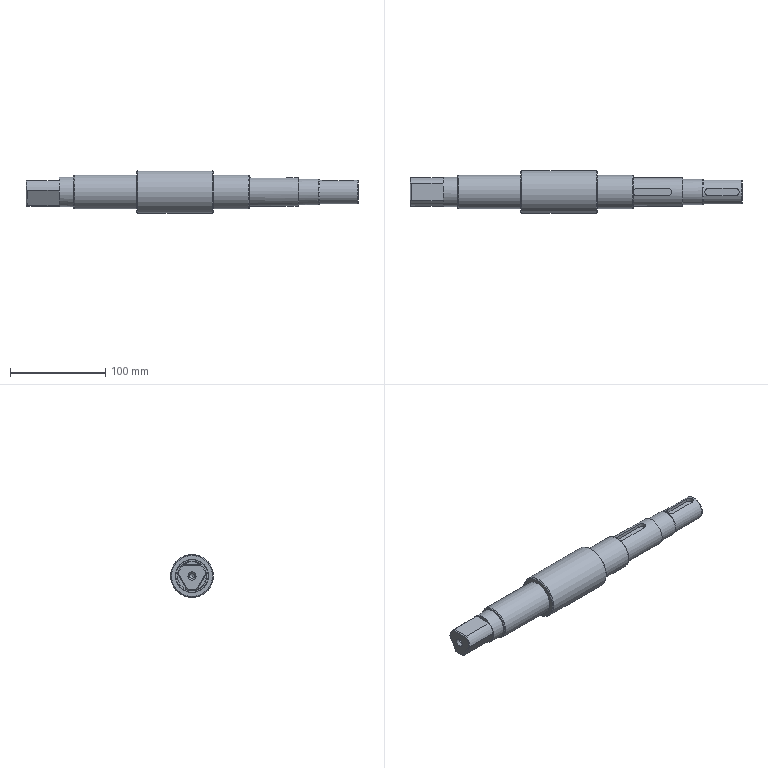NC program | NX | posted with a generic post | part box 348.4 x 45 x 45 mm
Whole program:
N10 G17 G21 G94 G90
(刀补4 , TOOL : D4)
N12 T04 M6
N14 G54
N16 G17 G0 G90 X104.872 Y0.433 B0. C0. S4500 M3
N18 G43 Z30. H4
N20 Z-6.508
N22 G94 G1 X102.135 Z-6.652 F1000.
N24 X101.983 Y0.386 Z-6.66
N26 X101.822 Y0.23 Z-6.672
N28 X101.758 Y0.016 Z-6.684
N30 X101.806 Y-0.203 Z-6.695
N32 X101.925 Y-0.347 Z-6.705
N34 X102.106 Y-0.433 Z-6.716
N36 X111.836 Z-7.225
N38 X111.853 Y-0.422 Z-7.226
N40 X112.036 Y-0.414 Z-7.236
N42 X112.09 Y-0.412 Z-7.239
N44 X112.197 Y-0.413 Z-7.245
N46 X112.295 Y-0.411 Z-7.25
N48 X112.388 Y-0.38 Z-7.255
N50 X112.463 Y-0.354 Z-7.259
N52 X112.485 Y-0.338 Z-7.26
N54 X112.533 Y-0.275 Z-7.265
N56 X112.592 Y-0.2 Z-7.27
N58 X112.638 Y0. Z-7.28
N60 X112.592 Y0.199 Z-7.291
N62 X112.534 Y0.274 Z-7.296
N64 X112.48 Y0.329 Z-7.3
N66 X112.429 Y0.365 Z-7.303
N68 X112.196 Y0.433 Z-7.316
N70 X107.299 Z-7.573
N72 G41 X107.2 Y0.45 D4
N74 X102.2 F1650.
N76 G3 X101.75 Y0. R0.45
N78 X102.2 Y-0.45 R0.45
N80 G1 X111.841
N82 X111.858 Y-0.439
N84 X112.037 Y-0.432
N86 X112.09 Y-0.43
N88 X112.198
N90 X112.299 Y-0.431
N92 X112.394 Y-0.396
N94 X112.457 Y-0.378
N96 X112.51 Y-0.34
N98 X112.547 Y-0.285
N100 G3 X112.547 Y0.285 R0.462
N102 G1 X112.491 Y0.342
N104 X112.437 Y0.381
N106 X112.201 Y0.45
N108 X107.2
N110 X103.512 Z-7.637
N112 X102.2
N114 G3 X101.75 Y0. R0.45
N116 X102.2 Y-0.45 R0.45
N118 G1 X111.841
N120 X111.858 Y-0.439
N122 X112.037 Y-0.432
N124 X112.09 Y-0.43
N126 X112.198
N128 X112.299 Y-0.431
N130 X112.394 Y-0.396
N132 X112.457 Y-0.378
N134 X112.51 Y-0.34
N136 X112.547 Y-0.285
N138 G3 X112.547 Y0.285 R0.462
N140 G1 X112.491 Y0.342
N142 X112.437 Y0.381
N144 X112.201 Y0.45
N146 X107.2
N148 X103.512 Z-7.701
N150 X102.2
N152 G3 X101.75 Y0. R0.45
N154 X102.2 Y-0.45 R0.45
N156 G1 X111.841
N158 X111.858 Y-0.439
N160 X112.037 Y-0.432
N162 X112.09 Y-0.43
N164 X112.198
N166 X112.299 Y-0.431
N168 X112.394 Y-0.396
N170 X112.457 Y-0.378
N172 X112.51 Y-0.34
N174 X112.547 Y-0.285
N176 G3 X112.547 Y0.285 R0.462
N178 G1 X112.491 Y0.342
N180 X112.437 Y0.381
N182 X112.201 Y0.45
N184 X107.2
N186 X103.512 Z-7.766
N188 X102.2
N190 G3 X101.75 Y0. R0.45
N192 X102.2 Y-0.45 R0.45
N194 G1 X111.841
N196 X111.858 Y-0.439
N198 X112.037 Y-0.431
N200 X112.09 Y-0.43
N202 X112.198
N204 X112.299 Y-0.431
N206 X112.394 Y-0.396
N208 X112.457 Y-0.378
N210 X112.51 Y-0.34
N212 X112.547 Y-0.285
N214 G3 X112.547 Y0.285 R0.462
N216 G1 X112.491 Y0.342
N218 X112.437 Y0.381
N220 X112.201 Y0.45
N222 X107.2
N224 X103.512 Z-7.83
N226 X102.2
N228 G3 X101.75 Y0. R0.45
N230 X102.2 Y-0.45 R0.45
N232 G1 X111.841
N234 X111.852 Y-0.432
N236 X111.873 Y-0.438
N238 X112.238 Y-0.431
N240 X112.394 Y-0.396
N242 X112.457 Y-0.378
N244 X112.51 Y-0.34
N246 X112.547 Y-0.285
N248 G3 X112.563 Y0.265 R0.467
N250 G1 X112.483 Y0.348
N252 X112.437 Y0.381
N254 X112.201 Y0.45
N256 X107.2
N258 X103.512 Z-7.895
N260 X102.2
N262 G3 X101.75 Y0. R0.45
N264 X102.2 Y-0.45 R0.45
N266 G1 X111.841
N268 X111.852 Y-0.432
N270 X111.873 Y-0.438
N272 X112.238 Y-0.431
N274 X112.394 Y-0.396
N276 G3 X112.594 Y-0.19 R0.308
N278 G1 X112.65 Y0.
N280 X112.578 Y0.242
N282 X112.491 Y0.342
N284 X112.437 Y0.381
N286 X112.201 Y0.45
N288 X107.2
N290 X103.512 Z-7.959
N292 X102.2
N294 G3 X101.75 Y0. R0.45
N296 X102.2 Y-0.45 R0.45
N298 G1 X111.841
N300 X111.852 Y-0.432
N302 X111.873 Y-0.438
N304 X112.238 Y-0.431
N306 X112.394 Y-0.396
N308 G3 X112.594 Y-0.19 R0.308
N310 G1 X112.65 Y0.
N312 X112.578 Y0.242
N314 X112.491 Y0.342
N316 X112.437 Y0.381
N318 X112.201 Y0.45
N320 X107.2
N322 X103.512 Z-8.023
N324 X102.2
N326 G3 X101.75 Y0. R0.45
N328 X102.2 Y-0.45 R0.45
N330 G1 X111.841
N332 X111.852 Y-0.432
N334 X111.873 Y-0.438
N336 X112.238 Y-0.431
N338 X112.394 Y-0.396
N340 G3 X112.594 Y-0.19 R0.308
N342 G1 X112.65 Y0.
N344 X112.578 Y0.242
N346 X112.491 Y0.342
N348 X112.437 Y0.381
N350 X112.201 Y0.45
N352 X107.2
N354 X103.512 Z-8.088
N356 X102.2
N358 G3 X101.75 Y0. R0.45
N360 X102.2 Y-0.45 R0.45
N362 G1 X111.841
N364 X111.852 Y-0.432
N366 X111.873 Y-0.438
N368 X112.238 Y-0.431
N370 X112.253 Y-0.429
N372 X112.394 Y-0.396
N374 G3 X112.594 Y-0.19 R0.308
N376 G1 X112.65 Y0.
N378 X112.578 Y0.242
N380 X112.571 Y0.254
N382 X112.483 Y0.348
N384 X112.437 Y0.381
N386 X112.201 Y0.45
N388 X107.2
N390 X103.512 Z-8.152
N392 X102.2
N394 G3 X101.75 Y0. R0.45
N396 X102.2 Y-0.45 R0.45
N398 G1 X111.874
N400 X111.876 Y-0.439
N402 X111.91 Y-0.437
N404 X112.238 Y-0.431
N406 X112.253 Y-0.429
N408 X112.394 Y-0.396
N410 G3 X112.594 Y-0.19 R0.308
N412 G1 X112.65 Y0.
N414 X112.578 Y0.242
N416 X112.571 Y0.254
N418 X112.483 Y0.348
N420 X112.437 Y0.381
N422 X112.201 Y0.45
N424 X107.2
N426 X103.512 Z-8.216
N428 X102.2
N430 G3 X101.75 Y0. R0.45
N432 X102.2 Y-0.45 R0.45
N434 G1 X111.911
N436 X111.912 Y-0.437
N438 X111.947 Y-0.435
N440 X112.238 Y-0.431
N442 X112.253 Y-0.429
N444 X112.394 Y-0.396
N446 G3 X112.594 Y-0.19 R0.308
N448 G1 X112.65 Y0.
N450 X112.578 Y0.242
N452 X112.571 Y0.254
N454 X112.483 Y0.348
N456 X112.437 Y0.381
N458 X112.201 Y0.45
N460 X107.2
N462 X103.512 Z-8.281
N464 X102.2
N466 G3 X101.75 Y0. R0.45
N468 X102.2 Y-0.45 R0.45
N470 G1 X111.947
N472 X111.983 Y-0.434
N474 X112.02 Y-0.432
N476 X112.238 Y-0.431
N478 X112.253 Y-0.429
N480 X112.394 Y-0.396
N482 G3 X112.594 Y-0.19 R0.308
N484 G1 X112.65 Y0.
N486 X112.578 Y0.242
N488 X112.483 Y0.348
N490 X112.437 Y0.381
N492 X112.201 Y0.45
N494 X107.2
N496 X103.512 Z-8.345
N498 X102.2
N500 G3 X101.75 Y0. R0.45
N502 X102.2 Y-0.45 R0.45
N504 G1 X111.984
N506 X112.034 Y-0.421
N508 X112.09 Y-0.429
N510 G3 X112.4 Y-0.394 R0.819
N512 X112.591 Y-0.2 R0.289
N514 G1 X112.65 Y0.
N516 X112.578 Y0.242
N518 X112.483 Y0.348
N520 X112.437 Y0.381
N522 X112.201 Y0.45
N524 X107.2
N526 X103.512 Z-8.41
N528 X102.2
N530 G3 X101.75 Y0. R0.45
N532 X102.2 Y-0.45 R0.45
N534 G1 X112.021
N536 X112.042 Y-0.423
N538 X112.076 Y-0.428
N540 G3 X112.4 Y-0.394 R0.819
N542 X112.591 Y-0.2 R0.289
N544 G1 X112.65 Y0.
N546 X112.578 Y0.242
N548 X112.483 Y0.348
N550 X112.437 Y0.381
N552 X112.201 Y0.45
N554 X107.2
N556 X103.512 Z-8.474
N558 X102.2
N560 G3 X101.75 Y0. R0.45
N562 X102.2 Y-0.45 R0.45
N564 G1 X112.057
N566 X112.056 Y-0.43
N568 X112.073 Y-0.419
N570 X112.09 Y-0.429
N572 G3 X112.4 Y-0.394 R0.818
N574 X112.591 Y-0.2 R0.289
N576 G1 X112.65 Y0.
N578 X112.578 Y0.242
N580 X112.483 Y0.348
N582 X112.437 Y0.381
N584 X112.201 Y0.45
N586 X107.2
N588 X103.512 Z-8.538
N590 X102.2
N592 G3 X101.75 Y0. R0.45
N594 X102.2 Y-0.45 R0.45
N596 G1 X112.073
N598 X112.09 Y-0.429
N600 G3 X112.4 Y-0.394 R0.818
N602 X112.591 Y-0.2 R0.289
N604 G1 X112.65 Y0.
N606 X112.578 Y0.242
N608 X112.483 Y0.348
N610 X112.437 Y0.381
N612 X112.201 Y0.45
N614 X107.2
N616 X103.512 Z-8.603
N618 X102.2
N620 G3 X101.75 Y0. R0.45
N622 X102.2 Y-0.45 R0.45
N624 G1 X112.073
N626 X112.09 Y-0.429
N628 G3 X112.404 Y-0.393 R0.783
N630 X112.591 Y-0.2 R0.288
N632 G1 X112.65 Y0.
N634 X112.578 Y0.242
N636 X112.483 Y0.348
N638 X112.437 Y0.381
N640 X112.201 Y0.45
N642 X107.2
N644 X103.512 Z-8.667
N646 X102.2
N648 G3 X101.75 Y0. R0.45
N650 X102.2 Y-0.45 R0.45
N652 G1 X112.073
N654 X112.09 Y-0.429
N656 G3 X112.404 Y-0.393 R0.783
N658 X112.591 Y-0.2 R0.288
N660 G1 X112.65 Y0.
N662 X112.578 Y0.242
N664 X112.483 Y0.348
N666 X112.437 Y0.381
N668 X112.201 Y0.45
N670 X107.2
N672 X103.512 Z-8.732
N674 X102.2
N676 G3 X101.75 Y0. R0.45
N678 X102.2 Y-0.45 R0.45
N680 G1 X112.073
N682 X112.09 Y-0.429
N684 X112.141 Y-0.411
N686 X112.195 Y-0.418
N688 X112.238 Y-0.45
N690 X112.233 Y-0.432
N692 X112.252 Y-0.43
N694 X112.394 Y-0.396
N696 G3 X112.594 Y-0.19 R0.308
N698 G1 X112.65 Y0.
N700 X112.578 Y0.242
N702 X112.483 Y0.348
N704 X112.437 Y0.381
N706 X112.201 Y0.45
N708 X107.2
N710 X103.512 Z-8.796
N712 X102.2
N714 G3 X101.75 Y0. R0.45
N716 X102.2 Y-0.45 R0.45
N718 G1 X112.073
N720 X112.09 Y-0.429
N722 X112.141 Y-0.41
N724 X112.195 Y-0.418
N726 X112.238 Y-0.45
N728 X112.233 Y-0.432
N730 X112.252 Y-0.429
N732 X112.394 Y-0.396
N734 G3 X112.594 Y-0.19 R0.308
N736 G1 X112.65 Y0.
N738 X112.578 Y0.242
N740 X112.483 Y0.348
N742 X112.437 Y0.381
N744 X112.201 Y0.45
N746 X107.2
N748 X103.512 Z-8.86
N750 X102.2
N752 G3 X101.75 Y0. R0.45
N754 X102.2 Y-0.45 R0.45
N756 G1 X112.073
N758 X112.09 Y-0.429
N760 X112.141 Y-0.41
N762 X112.195 Y-0.417
N764 X112.238 Y-0.45
N766 X112.233 Y-0.432
N768 X112.252 Y-0.429
N770 X112.394 Y-0.396
N772 G3 X112.594 Y-0.19 R0.308
N774 G1 X112.65 Y0.
N776 X112.578 Y0.242
N778 X112.483 Y0.348
N780 X112.437 Y0.381
N782 X112.201 Y0.45
N784 X107.2
N786 X103.512 Z-8.925
N788 X102.2
N790 G3 X101.75 Y0. R0.45
N792 X102.2 Y-0.45 R0.45
N794 G1 X112.073
N796 X112.09 Y-0.429
N798 X112.141 Y-0.41
N800 X112.195 Y-0.417
N802 X112.238 Y-0.45
N804 X112.233 Y-0.432
N806 X112.252 Y-0.429
N808 X112.394 Y-0.396
N810 G3 X112.594 Y-0.19 R0.308
N812 G1 X112.65 Y0.
N814 X112.578 Y0.242
N816 X112.483 Y0.348
N818 X112.437 Y0.381
N820 X112.201 Y0.45
N822 X107.2
N824 X103.512 Z-8.989
N826 X102.2
N828 G3 X101.75 Y0. R0.45
N830 X102.2 Y-0.45 R0.45
N832 G1 X112.073
N834 X112.09 Y-0.429
N836 X112.141 Y-0.41
N838 X112.195 Y-0.417
N840 X112.238 Y-0.45
N842 X112.233 Y-0.432
N844 X112.252 Y-0.429
N846 X112.379 Y-0.399
N848 X112.394 Y-0.396
N850 G3 X112.594 Y-0.19 R0.308
N852 G1 X112.65 Y0.
N854 X112.578 Y0.242
N856 X112.483 Y0.348
N858 X112.437 Y0.381
N860 X112.201 Y0.45
N862 X107.2
N864 X103.512 Z-9.053
N866 X102.2
N868 G3 X101.75 Y0. R0.45
N870 X102.2 Y-0.45 R0.45
N872 G1 X112.073
N874 X112.09 Y-0.429
N876 X112.141 Y-0.41
N878 X112.195 Y-0.417
N880 X112.238 Y-0.45
N882 X112.233 Y-0.432
N884 X112.252 Y-0.429
N886 X112.379 Y-0.399
N888 X112.398 Y-0.404
N890 G3 X112.2 Y0.45 R0.45
N892 G1 X107.2
N894 X103.512 Z-9.118
N896 X102.2
N898 G3 X101.75 Y0. R0.45
N900 X102.2 Y-0.45 R0.45
N902 G1 X112.073
N904 X112.09 Y-0.429
N906 X112.141 Y-0.41
N908 X112.195 Y-0.417
N910 X112.238 Y-0.45
N912 X112.233 Y-0.432
N914 X112.252 Y-0.429
N916 X112.379 Y-0.399
N918 X112.398 Y-0.404
N920 G3 X112.2 Y0.45 R0.45
N922 G1 X107.2
N924 X103.512 Z-9.182
N926 X102.2
N928 G3 X101.75 Y0. R0.45
N930 X102.2 Y-0.45 R0.45
N932 G1 X112.073
N934 X112.09 Y-0.429
N936 X112.141 Y-0.409
N938 X112.195 Y-0.417
N940 X112.238 Y-0.45
N942 X112.233 Y-0.432
N944 X112.252 Y-0.429
N946 X112.379 Y-0.399
N948 X112.398 Y-0.404
N950 G3 X112.2 Y0.45 R0.45
N952 G1 X107.2
N954 X103.512 Z-9.247
N956 X102.2
N958 G3 X101.75 Y0. R0.45
N960 X102.2 Y-0.45 R0.45
N962 G1 X112.073
N964 X112.09 Y-0.429
N966 X112.207 Y-0.43
N968 X112.222 Y-0.449
N970 X112.271 Y-0.444
N972 X112.28 Y-0.412
N974 X112.316 Y-0.403
N976 X112.34 Y-0.428
N978 G3 X112.2 Y0.45 R0.45
N980 G1 X107.2
N982 X103.512 Z-9.311
N984 X102.2
N986 G3 X101.75 Y0. R0.45
N988 X102.2 Y-0.45 R0.45
N990 G1 X112.073
N992 X112.09 Y-0.429
N994 X112.207 Y-0.43
N996 X112.222 Y-0.449
N998 X112.271 Y-0.444
N1000 X112.28 Y-0.412
N1002 X112.316 Y-0.403
N1004 X112.34 Y-0.428
N1006 G3 X112.2 Y0.45 R0.45
N1008 G1 X107.2
N1010 X103.512 Z-9.375
N1012 X102.2
N1014 G3 X101.75 Y0. R0.45
N1016 X102.2 Y-0.45 R0.45
N1018 G1 X112.073
N1020 X112.09 Y-0.429
N1022 X112.207 Y-0.43
N1024 X112.222 Y-0.449
N1026 X112.271 Y-0.444
N1028 X112.28 Y-0.412
N1030 X112.316 Y-0.403
N1032 X112.34 Y-0.428
N1034 G3 X112.2 Y0.45 R0.45
N1036 G1 X107.2
N1038 X103.512 Z-9.44
N1040 X102.2
N1042 G3 X101.75 Y0. R0.45
N1044 X102.2 Y-0.45 R0.45
N1046 G1 X112.073
N1048 X112.09 Y-0.429
N1050 X112.207 Y-0.43
N1052 X112.222 Y-0.449
N1054 X112.271 Y-0.444
N1056 X112.28 Y-0.412
N1058 X112.316 Y-0.403
N1060 X112.34 Y-0.428
N1062 G3 X112.2 Y0.45 R0.45
N1064 G1 X107.2
N1066 X103.512 Z-9.504
N1068 X102.2
N1070 G3 X101.75 Y0. R0.45
N1072 X102.2 Y-0.45 R0.45
N1074 G1 X112.073
N1076 X112.09 Y-0.429
N1078 X112.207 Y-0.43
N1080 X112.222 Y-0.449
N1082 X112.271 Y-0.444
N1084 X112.28 Y-0.411
N1086 X112.316 Y-0.403
N1088 X112.34 Y-0.428
N1090 G3 X112.2 Y0.45 R0.45
N1092 G1 X107.2
N1094 X103.512 Z-9.569
N1096 X102.2
N1098 G3 X101.75 Y0. R0.45
N1100 X102.2 Y-0.45 R0.45
N1102 G1 X112.073
N1104 X112.09 Y-0.429
N1106 X112.207
N1108 X112.222 Y-0.449
N1110 X112.271 Y-0.444
N1112 X112.28 Y-0.411
N1114 X112.316 Y-0.403
N1116 X112.34 Y-0.428
N1118 G3 X112.2 Y0.45 R0.45
N1120 G1 X107.2
N1122 X103.512 Z-9.633
N1124 X102.2
N1126 G3 X101.75 Y0. R0.45
N1128 X102.2 Y-0.45 R0.45
N1130 G1 X112.073
N1132 X112.09 Y-0.429
N1134 X112.207
N1136 X112.222 Y-0.449
N1138 X112.271 Y-0.444
N1140 X112.28 Y-0.411
N1142 X112.316 Y-0.403
N1144 X112.34 Y-0.428
N1146 G3 X112.2 Y0.45 R0.45
N1148 G1 X107.2
N1150 X103.512 Z-9.697
N1152 X102.2
N1154 G3 X101.75 Y0. R0.45
N1156 X102.2 Y-0.45 R0.45
N1158 G1 X112.073
N1160 X112.09 Y-0.429
N1162 X112.207
N1164 X112.222 Y-0.449
N1166 X112.271 Y-0.444
N1168 X112.28 Y-0.411
N1170 X112.316 Y-0.403
N1172 X112.34 Y-0.428
N1174 G3 X112.2 Y0.45 R0.45
N1176 G1 X107.2
N1178 X103.512 Z-9.762
N1180 X102.2
N1182 G3 X101.75 Y0. R0.45
N1184 X102.2 Y-0.45 R0.45
N1186 G1 X112.073
N1188 X112.09 Y-0.429
N1190 X112.207
N1192 X112.222 Y-0.449
N1194 X112.271 Y-0.444
N1196 X112.28 Y-0.411
N1198 X112.316 Y-0.403
N1200 X112.34 Y-0.428
N1202 G3 X112.2 Y0.45 R0.45
N1204 G1 X107.2
N1206 X103.512 Z-9.826
N1208 X102.2
N1210 G3 X101.75 Y0. R0.45
N1212 X102.2 Y-0.45 R0.45
N1214 G1 X112.073
N1216 X112.09 Y-0.429
N1218 X112.207
N1220 X112.222 Y-0.449
N1222 X112.271 Y-0.444
N1224 X112.28 Y-0.411
N1226 X112.316 Y-0.403
N1228 X112.34 Y-0.428
N1230 G3 X112.2 Y0.45 R0.45
N1232 G1 X107.2
N1234 X103.512 Z-9.89
N1236 X102.2
N1238 G3 X101.75 Y0. R0.45
N1240 X102.2 Y-0.45 R0.45
N1242 G1 X112.073
N1244 X112.09 Y-0.429
N1246 X112.207
N1248 X112.222 Y-0.449
N1250 X112.271 Y-0.444
N1252 X112.28 Y-0.411
N1254 X112.316 Y-0.403
N1256 X112.34 Y-0.428
N1258 G3 X112.2 Y0.45 R0.45
N1260 G1 X107.2
N1262 X103.512 Z-9.955
N1264 X102.2
N1266 G3 X101.75 Y0. R0.45
N1268 X102.2 Y-0.45 R0.45
N1270 G1 X112.073
N1272 X112.09 Y-0.429
N1274 X112.207
N1276 X112.222 Y-0.449
N1278 X112.271 Y-0.444
N1280 X112.28 Y-0.411
N1282 X112.316 Y-0.403
N1284 X112.34 Y-0.428
N1286 G3 X112.2 Y0.45 R0.45
N1288 G1 X107.2
N1290 X103.512 Z-10.019
N1292 X102.2
N1294 G3 X101.75 Y0. R0.45
N1296 X102.2 Y-0.45 R0.45
N1298 G1 X112.073
N1300 X112.09 Y-0.429
N1302 X112.207
N1304 X112.222 Y-0.449
N1306 X112.271 Y-0.444
N1308 X112.28 Y-0.411
N1310 X112.316 Y-0.403
N1312 X112.34 Y-0.428
N1314 G3 X112.2 Y0.45 R0.45
N1316 G1 X107.2
N1318 X103.512 Z-10.084
N1320 X102.2
N1322 G3 X101.75 Y0. R0.45
N1324 X102.2 Y-0.45 R0.45
N1326 G1 X112.073
N1328 X112.09 Y-0.429
N1330 X112.207
N1332 X112.222 Y-0.449
N1334 X112.271 Y-0.444
N1336 X112.28 Y-0.411
N1338 X112.316 Y-0.403
N1340 X112.34 Y-0.428
N1342 G3 X112.2 Y0.45 R0.45
N1344 G1 X107.2
N1346 X103.512 Z-10.148
N1348 X102.2
N1350 G3 X101.75 Y0. R0.45
N1352 X102.2 Y-0.45 R0.45
N1354 G1 X112.073
N1356 X112.09 Y-0.429
N1358 X112.207
N1360 X112.222 Y-0.449
N1362 X112.271 Y-0.444
N1364 X112.28 Y-0.411
N1366 X112.316 Y-0.403
N1368 X112.34 Y-0.428
N1370 G3 X112.2 Y0.45 R0.45
N1372 G1 X107.2
N1374 X103.512 Z-10.212
N1376 X102.2
N1378 G3 X101.75 Y0. R0.45
N1380 X102.2 Y-0.45 R0.45
N1382 G1 X112.073
N1384 X112.09 Y-0.429
N1386 X112.207
N1388 X112.222 Y-0.449
N1390 X112.271 Y-0.444
N1392 X112.28 Y-0.411
N1394 X112.316 Y-0.402
N1396 X112.34 Y-0.428
N1398 G3 X112.2 Y0.45 R0.45
N1400 G1 X107.2
N1402 X103.512 Z-10.277
N1404 X102.2
N1406 G3 X101.75 Y0. R0.45
N1408 X102.2 Y-0.45 R0.45
N1410 G1 X112.073
N1412 X112.09 Y-0.429
N1414 X112.207
N1416 X112.222 Y-0.449
N1418 X112.271 Y-0.444
N1420 X112.28 Y-0.411
N1422 X112.316 Y-0.402
N1424 X112.34 Y-0.428
N1426 G3 X112.2 Y0.45 R0.45
N1428 G1 X107.2
N1430 X103.512 Z-10.341
N1432 X102.2
N1434 G3 X101.75 Y0. R0.45
N1436 X102.2 Y-0.45 R0.45
N1438 G1 X112.073
N1440 X112.09 Y-0.429
N1442 X112.207
N1444 X112.222 Y-0.449
N1446 X112.271 Y-0.444
N1448 X112.28 Y-0.411
N1450 X112.316 Y-0.402
N1452 X112.34 Y-0.428
N1454 G3 X112.2 Y0.45 R0.45
N1456 G1 X107.2
N1458 X103.512 Z-10.405
N1460 X102.2
N1462 G3 X101.75 Y0. R0.45
N1464 X102.2 Y-0.45 R0.45
N1466 G1 X112.055
N1468 Y-0.43
N1470 X112.072 Y-0.419
N1472 X112.09 Y-0.429
N1474 X112.207
N1476 X112.222 Y-0.449
N1478 X112.271 Y-0.444
N1480 X112.28 Y-0.411
N1482 X112.316 Y-0.402
N1484 X112.34 Y-0.428
N1486 G3 X112.2 Y0.45 R0.45
N1488 G1 X107.2
N1490 X103.512 Z-10.47
N1492 X102.2
N1494 G3 X101.75 Y0. R0.45
N1496 X102.2 Y-0.45 R0.45
N1498 G1 X112.055
N1500 Y-0.43
N1502 X112.072 Y-0.419
N1504 X112.09 Y-0.429
N1506 X112.207
N1508 X112.222 Y-0.449
N1510 X112.271 Y-0.444
N1512 X112.28 Y-0.411
N1514 X112.316 Y-0.402
N1516 X112.34 Y-0.428
N1518 G3 X112.2 Y0.45 R0.45
N1520 G1 X107.2
N1522 X103.512 Z-10.534
N1524 X102.2
N1526 G3 X101.75 Y0. R0.45
N1528 X102.2 Y-0.45 R0.45
N1530 G1 X112.055
N1532 Y-0.43
N1534 X112.072 Y-0.419
N1536 X112.09 Y-0.429
N1538 X112.207
N1540 X112.222 Y-0.449
N1542 X112.271 Y-0.444
N1544 X112.28 Y-0.411
N1546 X112.316 Y-0.402
N1548 X112.34 Y-0.428
N1550 G3 X112.2 Y0.45 R0.45
N1552 G1 X107.2
N1554 X103.512 Z-10.599
N1556 X102.2
N1558 G3 X101.75 Y0. R0.45
N1560 X102.2 Y-0.45 R0.45
N1562 G1 X112.055
N1564 Y-0.43
N1566 X112.072 Y-0.419
N1568 X112.09 Y-0.429
N1570 X112.207
N1572 X112.222 Y-0.449
N1574 X112.271 Y-0.444
N1576 X112.28 Y-0.411
N1578 X112.316 Y-0.402
N1580 X112.34 Y-0.428
N1582 G3 X112.2 Y0.45 R0.45
N1584 G1 X107.2
N1586 X103.512 Z-10.663
N1588 X102.2
N1590 G3 X101.75 Y0. R0.45
N1592 X102.2 Y-0.45 R0.45
N1594 G1 X112.055
N1596 Y-0.43
N1598 X112.072 Y-0.419
N1600 X112.09 Y-0.429
N1602 X112.207
N1604 X112.222 Y-0.449
N1606 X112.271 Y-0.444
N1608 X112.28 Y-0.411
N1610 X112.316 Y-0.402
N1612 X112.34 Y-0.428
N1614 G3 X112.2 Y0.45 R0.45
N1616 G1 X107.2
N1618 X103.512 Z-10.727
N1620 X102.2
N1622 G3 X101.75 Y0. R0.45
N1624 X102.2 Y-0.45 R0.45
N1626 G1 X112.055
N1628 Y-0.43
N1630 X112.072 Y-0.419
N1632 X112.09 Y-0.429
N1634 X112.207
N1636 X112.222 Y-0.449
N1638 X112.271 Y-0.444
N1640 X112.28 Y-0.411
N1642 X112.316 Y-0.402
N1644 X112.34 Y-0.428
N1646 G3 X112.2 Y0.45 R0.45
N1648 G1 X107.2
N1650 X103.512 Z-10.792
N1652 X102.2
N1654 G3 X101.75 Y0. R0.45
N1656 X102.2 Y-0.45 R0.45
N1658 G1 X112.055
N1660 Y-0.43
N1662 X112.072 Y-0.419
N1664 X112.09 Y-0.429
N1666 X112.207
N1668 X112.222 Y-0.449
N1670 X112.271 Y-0.444
N1672 X112.28 Y-0.411
N1674 X112.316 Y-0.402
N1676 X112.34 Y-0.428
N1678 G3 X112.2 Y0.45 R0.45
N1680 G1 X107.2
N1682 X103.512 Z-10.856
N1684 X102.2
N1686 G3 X101.75 Y0. R0.45
N1688 X102.2 Y-0.45 R0.45
N1690 G1 X112.055
N1692 Y-0.43
N1694 X112.072 Y-0.419
N1696 X112.09 Y-0.428
N1698 X112.207 Y-0.429
N1700 X112.222 Y-0.449
N1702 X112.271 Y-0.444
N1704 X112.28 Y-0.411
N1706 X112.316 Y-0.402
N1708 X112.34 Y-0.428
N1710 G3 X112.2 Y0.45 R0.45
N1712 G1 X107.2
N1714 X103.512 Z-10.921
N1716 X102.2
N1718 G3 X101.75 Y0. R0.45
N1720 X102.2 Y-0.45 R0.45
N1722 G1 X112.055
N1724 Y-0.43
N1726 X112.072 Y-0.419
N1728 X112.09 Y-0.428
N1730 X112.207 Y-0.429
N1732 X112.222 Y-0.449
N1734 X112.271 Y-0.444
N1736 X112.28 Y-0.411
N1738 X112.316 Y-0.402
N1740 X112.34 Y-0.428
N1742 G3 X112.2 Y0.45 R0.45
N1744 G1 X107.2
N1746 X103.512 Z-10.985
N1748 X102.2
N1750 G3 X101.75 Y0. R0.45
N1752 X102.2 Y-0.45 R0.45
N1754 G1 X112.055
N1756 Y-0.43
N1758 X112.072 Y-0.419
N1760 X112.09 Y-0.428
N1762 X112.207 Y-0.429
N1764 X112.222 Y-0.449
N1766 X112.271 Y-0.444
N1768 X112.28 Y-0.411
N1770 X112.316 Y-0.402
N1772 X112.34 Y-0.428
N1774 G3 X112.2 Y0.45 R0.45
N1776 G1 X107.2
N1778 X103.512 Z-11.049
N1780 X102.2
N1782 G3 X101.75 Y0. R0.45
N1784 X102.2 Y-0.45 R0.45
N1786 G1 X112.055
N1788 X112.053 Y-0.428
N1790 X112.075
N1792 X112.207
N1794 X112.222 Y-0.449
N1796 X112.271 Y-0.444
N1798 X112.28 Y-0.411
N1800 X112.316 Y-0.402
N1802 X112.34 Y-0.428
N1804 G3 X112.2 Y0.45 R0.45
N1806 G1 X107.2
N1808 X103.512 Z-11.114
N1810 X102.2
N1812 G3 X101.75 Y0. R0.45
N1814 X102.2 Y-0.45 R0.45
N1816 G1 X112.055
N1818 X112.053 Y-0.428
N1820 X112.075
N1822 X112.207
N1824 X112.222 Y-0.449
N1826 X112.271 Y-0.444
N1828 X112.28 Y-0.411
N1830 X112.316 Y-0.402
N1832 X112.34 Y-0.428
N1834 G3 X112.2 Y0.45 R0.45
N1836 G1 X107.2
N1838 X103.512 Z-11.178
N1840 X102.2
N1842 G3 X101.75 Y0. R0.45
N1844 X102.2 Y-0.45 R0.45
N1846 G1 X112.055
N1848 X112.053 Y-0.428
N1850 X112.075
N1852 X112.207
N1854 X112.222 Y-0.449
N1856 X112.271 Y-0.444
N1858 X112.28 Y-0.411
N1860 X112.316 Y-0.402
N1862 X112.34 Y-0.428
N1864 G3 X112.2 Y0.45 R0.45
N1866 G1 X107.2
N1868 X103.512 Z-11.242
N1870 X102.2
N1872 G3 X101.75 Y0. R0.45
N1874 X102.2 Y-0.45 R0.45
N1876 G1 X112.055
N1878 X112.053 Y-0.428
N1880 X112.075
N1882 X112.207
N1884 X112.222 Y-0.449
N1886 X112.255 Y-0.447
N1888 X112.271 Y-0.412
N1890 X112.311 Y-0.403
N1892 X112.34 Y-0.428
N1894 G3 X112.2 Y0.45 R0.45
N1896 G1 X107.2
N1898 X103.512 Z-11.307
N1900 X102.2
N1902 G3 X101.75 Y0. R0.45
N1904 X102.2 Y-0.45 R0.45
N1906 G1 X112.055
N1908 X112.053 Y-0.428
N1910 X112.075
N1912 X112.207
N1914 X112.222 Y-0.449
N1916 X112.255 Y-0.447
N1918 X112.271 Y-0.412
N1920 X112.311 Y-0.403
N1922 X112.34 Y-0.428
N1924 G3 X112.2 Y0.45 R0.45
N1926 G1 X107.2
N1928 X103.512 Z-11.371
N1930 X102.2
N1932 G3 X101.75 Y0. R0.45
N1934 X102.2 Y-0.45 R0.45
N1936 G1 X112.055
N1938 X112.053 Y-0.428
N1940 X112.075
N1942 X112.207
N1944 X112.222 Y-0.449
N1946 X112.255 Y-0.447
N1948 X112.27 Y-0.41
N1950 X112.311 Y-0.4
N1952 X112.34 Y-0.428
N1954 G3 X112.2 Y0.45 R0.45
N1956 G1 X107.2
N1958 X103.512 Z-11.436
N1960 X102.2
N1962 G3 X101.75 Y0. R0.45
N1964 X102.2 Y-0.45 R0.45
N1966 G1 X112.037
N1968 X112.088 Y-0.417
N1970 X112.149 Y-0.409
N1972 X112.207 Y-0.428
N1974 X112.222 Y-0.449
N1976 X112.255 Y-0.447
N1978 X112.27 Y-0.409
N1980 X112.311 Y-0.4
N1982 X112.34 Y-0.428
N1984 G3 X112.2 Y0.45 R0.45
N1986 G1 X107.2
N1988 X103.512 Z-11.5
N1990 X102.2
N1992 G3 X101.75 Y0. R0.45
N1994 X102.2 Y-0.45 R0.45
N1996 G1 X112.019
N1998 X112.017 Y-0.428
N2000 X112.04
N2002 X112.221
N2004 X112.235 Y-0.424
N2006 X112.244 Y-0.435
N2008 X112.238 Y-0.448
N2010 X112.255 Y-0.447
N2012 X112.276 Y-0.409
N2014 X112.319 Y-0.398
N2016 X112.355 Y-0.422
N2018 G3 X112.2 Y0.45 R0.45
N2020 G1 X103.512
N2022 G40
N2024 X103.413 Y0.433
N2026 Z-10.5
N2028 G0 Z30.
N2030 M5
N2032 M2